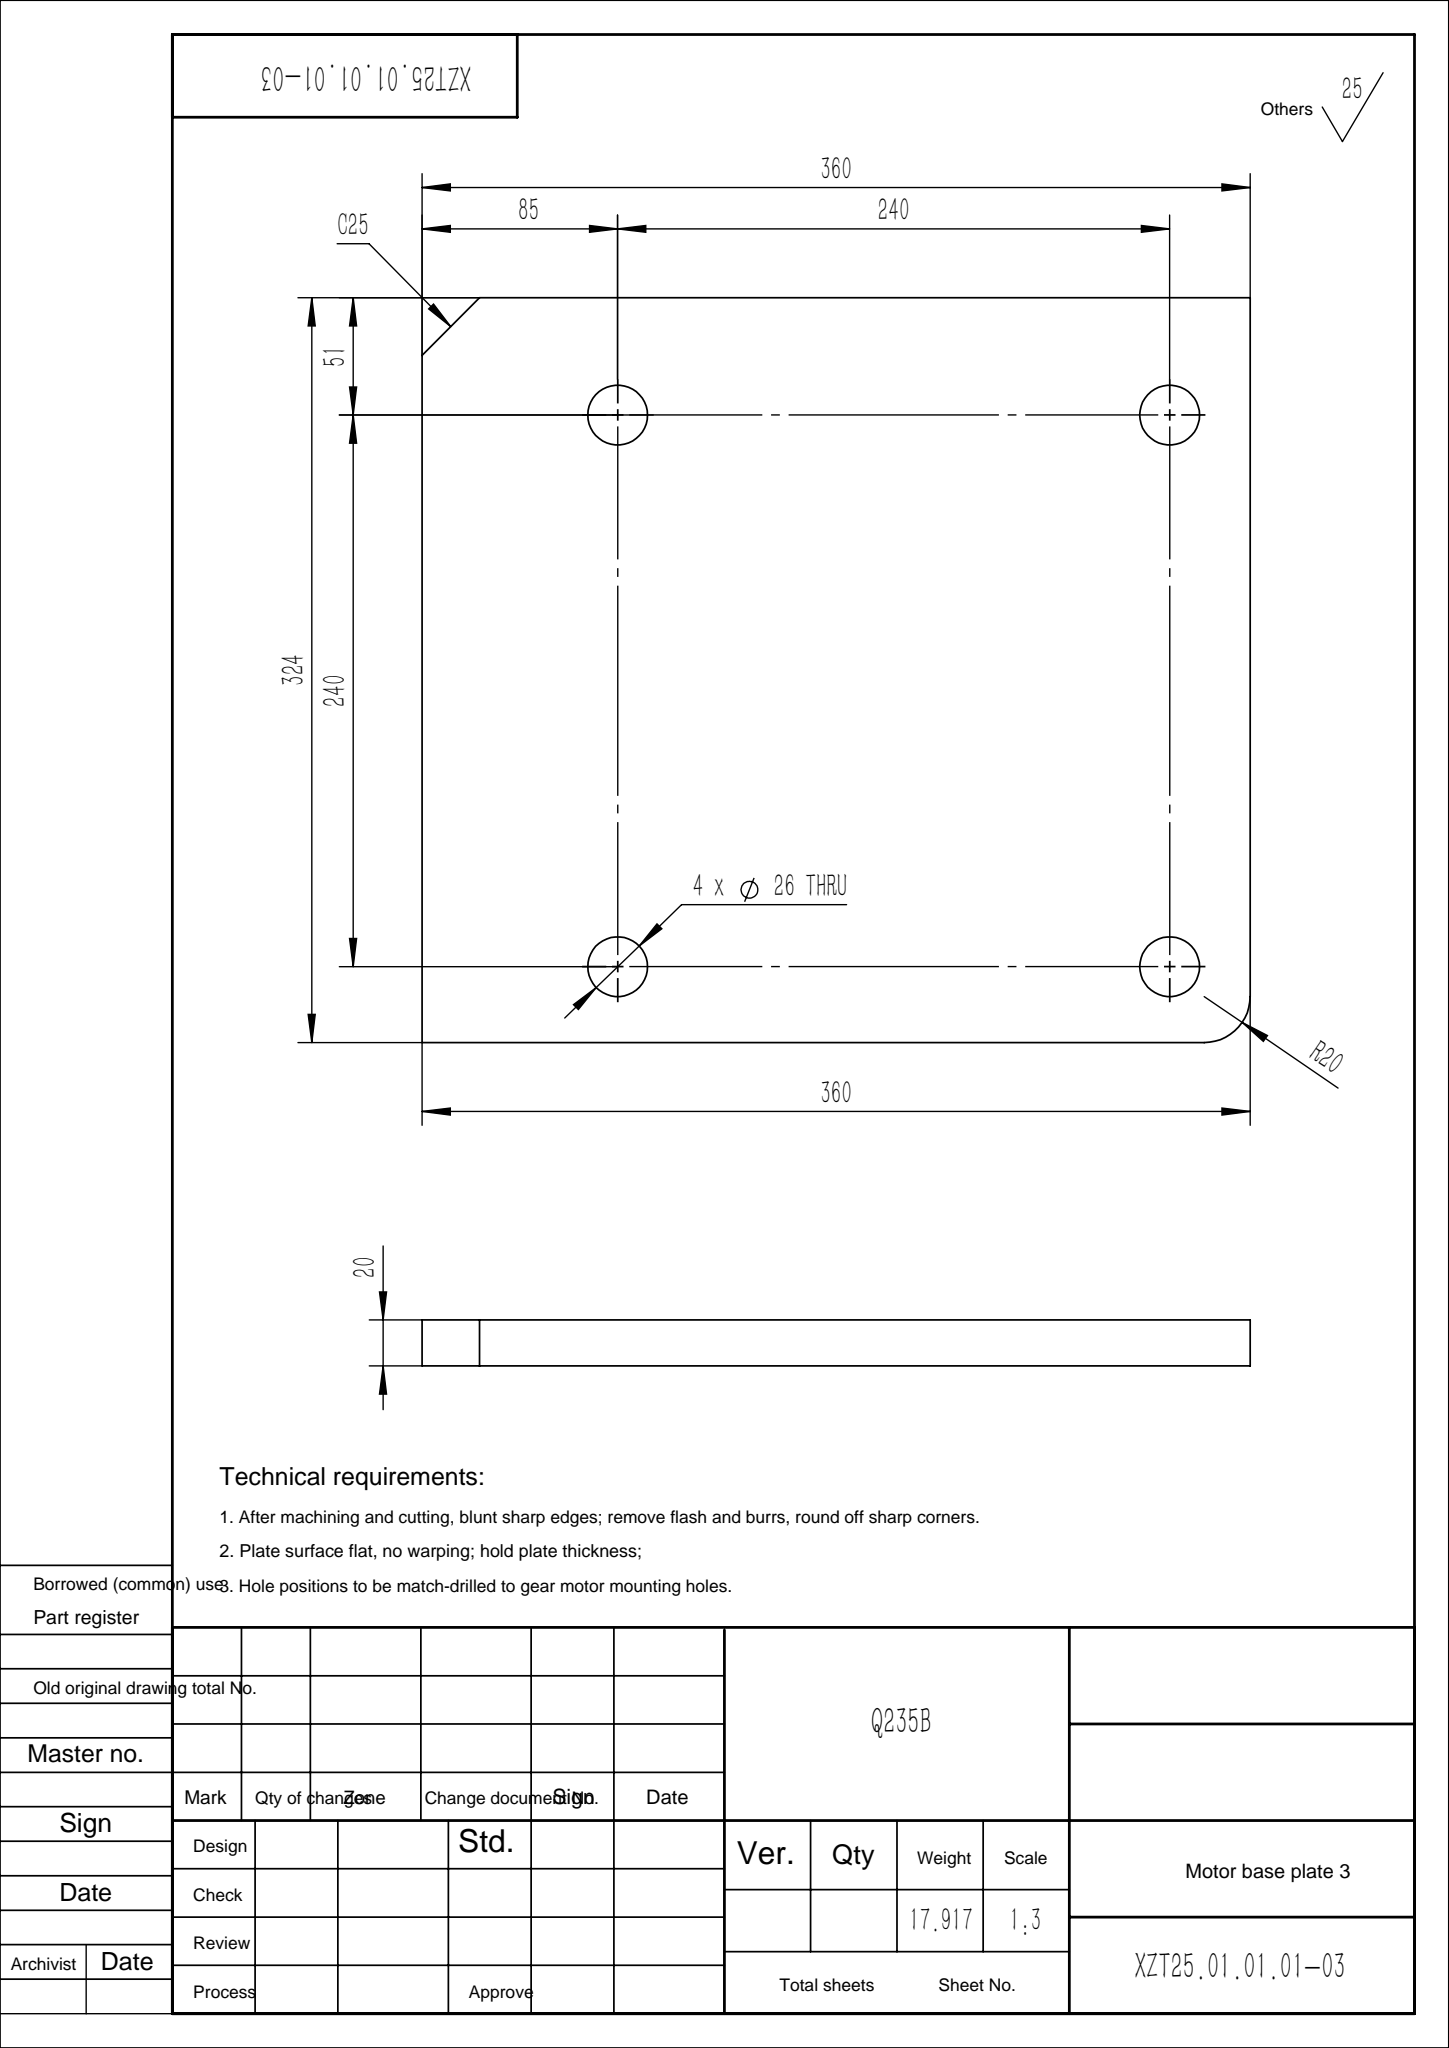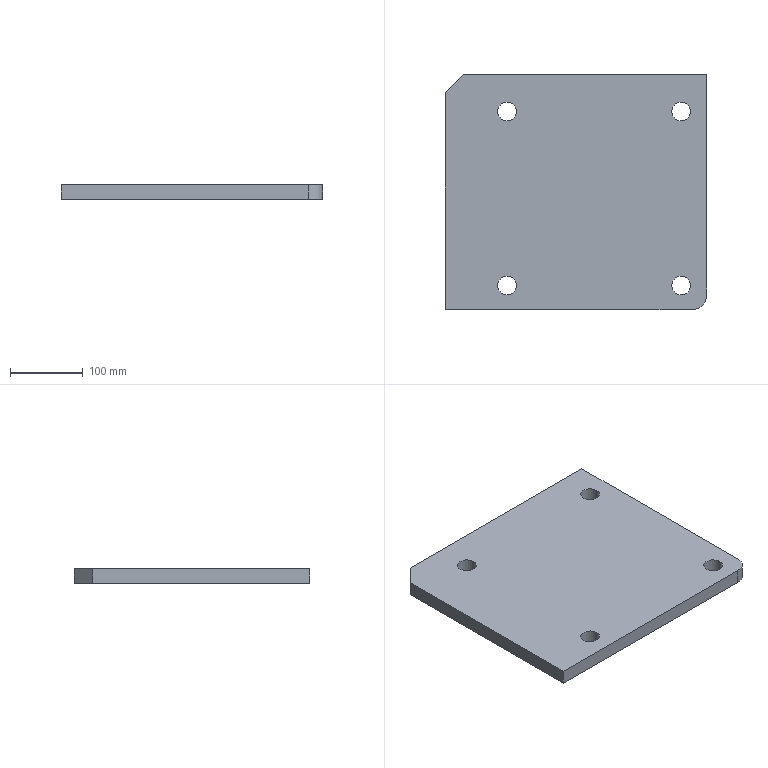Part | SolidWorks | features Chamfer 1, Extrusion 1, Fillet 1, HoleWzd 1 | 1 solid | 16 faces | box 360 x 324 x 20 mm | volume 2282359 mm3 | cylinder 9 | plane 7 | commonest cylinder face diameters 26 x8 40 x1
STEP:
#1=CARTESIAN_POINT('',(98.,33.,-10.));
#2=VERTEX_POINT('',#1);
#3=CARTESIAN_POINT('',(72.,33.,-10.));
#4=VERTEX_POINT('',#3);
#5=CARTESIAN_POINT('',(85.,33.,-10.));
#6=DIRECTION('',(0.,0.,-1.));
#7=DIRECTION('',(-1.,0.,0.));
#8=AXIS2_PLACEMENT_3D('',#5,#6,#7);
#9=CIRCLE('',#8,13.);
#10=EDGE_CURVE('',#2,#4,#9,.T.);
#11=ORIENTED_EDGE('',*,*,#10,.T.);
#12=CARTESIAN_POINT('',(72.,33.,10.));
#13=VERTEX_POINT('',#12);
#14=CARTESIAN_POINT('',(72.,33.,10.));
#15=DIRECTION('',(0.,0.,1.));
#16=VECTOR('',#15,1000.);
#17=LINE('',#14,#16);
#18=EDGE_CURVE('',#4,#13,#17,.T.);
#19=ORIENTED_EDGE('',*,*,#18,.T.);
#20=CARTESIAN_POINT('',(98.,33.,10.));
#21=VERTEX_POINT('',#20);
#22=CARTESIAN_POINT('',(85.,33.,10.));
#23=DIRECTION('',(0.,0.,1.));
#24=DIRECTION('',(1.,0.,0.));
#25=AXIS2_PLACEMENT_3D('',#22,#23,#24);
#26=CIRCLE('',#25,13.);
#27=EDGE_CURVE('',#13,#21,#26,.T.);
#28=ORIENTED_EDGE('',*,*,#27,.T.);
#29=CARTESIAN_POINT('',(98.,33.,10.));
#30=DIRECTION('',(0.,0.,1.));
#31=VECTOR('',#30,1000.);
#32=LINE('',#29,#31);
#33=EDGE_CURVE('',#2,#21,#32,.T.);
#34=ORIENTED_EDGE('',*,*,#33,.F.);
#35=EDGE_LOOP('',(#11,#19,#28,#34));
#36=FACE_OUTER_BOUND('',#35,.T.);
#37=CARTESIAN_POINT('',(85.,33.,10.));
#38=DIRECTION('',(0.,0.,1.));
#39=DIRECTION('',(1.,0.,0.));
#40=AXIS2_PLACEMENT_3D('',#37,#38,#39);
#41=CYLINDRICAL_SURFACE('',#40,13.);
#42=ADVANCED_FACE('',(#36),#41,.F.);
#43=CARTESIAN_POINT('',(338.,33.,-10.));
#44=VERTEX_POINT('',#43);
#45=CARTESIAN_POINT('',(312.,33.,-10.));
#46=VERTEX_POINT('',#45);
#47=CARTESIAN_POINT('',(325.,33.,-10.));
#48=DIRECTION('',(0.,0.,-1.));
#49=DIRECTION('',(-1.,0.,0.));
#50=AXIS2_PLACEMENT_3D('',#47,#48,#49);
#51=CIRCLE('',#50,13.);
#52=EDGE_CURVE('',#44,#46,#51,.T.);
#53=ORIENTED_EDGE('',*,*,#52,.T.);
#54=CARTESIAN_POINT('',(312.,33.,10.));
#55=VERTEX_POINT('',#54);
#56=CARTESIAN_POINT('',(312.,33.,10.));
#57=DIRECTION('',(0.,0.,1.));
#58=VECTOR('',#57,1000.);
#59=LINE('',#56,#58);
#60=EDGE_CURVE('',#46,#55,#59,.T.);
#61=ORIENTED_EDGE('',*,*,#60,.T.);
#62=CARTESIAN_POINT('',(338.,33.,10.));
#63=VERTEX_POINT('',#62);
#64=CARTESIAN_POINT('',(325.,33.,10.));
#65=DIRECTION('',(0.,0.,1.));
#66=DIRECTION('',(1.,0.,0.));
#67=AXIS2_PLACEMENT_3D('',#64,#65,#66);
#68=CIRCLE('',#67,13.);
#69=EDGE_CURVE('',#55,#63,#68,.T.);
#70=ORIENTED_EDGE('',*,*,#69,.T.);
#71=CARTESIAN_POINT('',(338.,33.,10.));
#72=DIRECTION('',(0.,0.,1.));
#73=VECTOR('',#72,1000.);
#74=LINE('',#71,#73);
#75=EDGE_CURVE('',#44,#63,#74,.T.);
#76=ORIENTED_EDGE('',*,*,#75,.F.);
#77=EDGE_LOOP('',(#53,#61,#70,#76));
#78=FACE_OUTER_BOUND('',#77,.T.);
#79=CARTESIAN_POINT('',(325.,33.,10.));
#80=DIRECTION('',(0.,0.,1.));
#81=DIRECTION('',(1.,0.,0.));
#82=AXIS2_PLACEMENT_3D('',#79,#80,#81);
#83=CYLINDRICAL_SURFACE('',#82,13.);
#84=ADVANCED_FACE('',(#78),#83,.F.);
#85=CARTESIAN_POINT('',(338.,273.,-10.));
#86=VERTEX_POINT('',#85);
#87=CARTESIAN_POINT('',(312.,273.,-10.));
#88=VERTEX_POINT('',#87);
#89=CARTESIAN_POINT('',(325.,273.,-10.));
#90=DIRECTION('',(0.,0.,-1.));
#91=DIRECTION('',(-1.,0.,0.));
#92=AXIS2_PLACEMENT_3D('',#89,#90,#91);
#93=CIRCLE('',#92,13.);
#94=EDGE_CURVE('',#86,#88,#93,.T.);
#95=ORIENTED_EDGE('',*,*,#94,.T.);
#96=CARTESIAN_POINT('',(312.,273.,10.));
#97=VERTEX_POINT('',#96);
#98=CARTESIAN_POINT('',(312.,273.,10.));
#99=DIRECTION('',(0.,0.,1.));
#100=VECTOR('',#99,1000.);
#101=LINE('',#98,#100);
#102=EDGE_CURVE('',#88,#97,#101,.T.);
#103=ORIENTED_EDGE('',*,*,#102,.T.);
#104=CARTESIAN_POINT('',(338.,273.,10.));
#105=VERTEX_POINT('',#104);
#106=CARTESIAN_POINT('',(325.,273.,10.));
#107=DIRECTION('',(0.,0.,1.));
#108=DIRECTION('',(1.,0.,0.));
#109=AXIS2_PLACEMENT_3D('',#106,#107,#108);
#110=CIRCLE('',#109,13.);
#111=EDGE_CURVE('',#97,#105,#110,.T.);
#112=ORIENTED_EDGE('',*,*,#111,.T.);
#113=CARTESIAN_POINT('',(338.,273.,10.));
#114=DIRECTION('',(0.,0.,1.));
#115=VECTOR('',#114,1000.);
#116=LINE('',#113,#115);
#117=EDGE_CURVE('',#86,#105,#116,.T.);
#118=ORIENTED_EDGE('',*,*,#117,.F.);
#119=EDGE_LOOP('',(#95,#103,#112,#118));
#120=FACE_OUTER_BOUND('',#119,.T.);
#121=CARTESIAN_POINT('',(325.,273.,10.));
#122=DIRECTION('',(0.,0.,1.));
#123=DIRECTION('',(1.,0.,0.));
#124=AXIS2_PLACEMENT_3D('',#121,#122,#123);
#125=CYLINDRICAL_SURFACE('',#124,13.);
#126=ADVANCED_FACE('',(#120),#125,.F.);
#127=CARTESIAN_POINT('',(98.,273.,-10.));
#128=VERTEX_POINT('',#127);
#129=CARTESIAN_POINT('',(72.,273.,-10.));
#130=VERTEX_POINT('',#129);
#131=CARTESIAN_POINT('',(85.,273.,-10.));
#132=DIRECTION('',(0.,0.,-1.));
#133=DIRECTION('',(-1.,0.,0.));
#134=AXIS2_PLACEMENT_3D('',#131,#132,#133);
#135=CIRCLE('',#134,13.);
#136=EDGE_CURVE('',#128,#130,#135,.T.);
#137=ORIENTED_EDGE('',*,*,#136,.T.);
#138=CARTESIAN_POINT('',(72.,273.,10.));
#139=VERTEX_POINT('',#138);
#140=CARTESIAN_POINT('',(72.,273.,10.));
#141=DIRECTION('',(0.,0.,1.));
#142=VECTOR('',#141,1000.);
#143=LINE('',#140,#142);
#144=EDGE_CURVE('',#130,#139,#143,.T.);
#145=ORIENTED_EDGE('',*,*,#144,.T.);
#146=CARTESIAN_POINT('',(98.,273.,10.));
#147=VERTEX_POINT('',#146);
#148=CARTESIAN_POINT('',(85.,273.,10.));
#149=DIRECTION('',(0.,0.,1.));
#150=DIRECTION('',(1.,0.,0.));
#151=AXIS2_PLACEMENT_3D('',#148,#149,#150);
#152=CIRCLE('',#151,13.);
#153=EDGE_CURVE('',#139,#147,#152,.T.);
#154=ORIENTED_EDGE('',*,*,#153,.T.);
#155=CARTESIAN_POINT('',(98.,273.,10.));
#156=DIRECTION('',(0.,0.,1.));
#157=VECTOR('',#156,1000.);
#158=LINE('',#155,#157);
#159=EDGE_CURVE('',#128,#147,#158,.T.);
#160=ORIENTED_EDGE('',*,*,#159,.F.);
#161=EDGE_LOOP('',(#137,#145,#154,#160));
#162=FACE_OUTER_BOUND('',#161,.T.);
#163=CARTESIAN_POINT('',(85.,273.,10.));
#164=DIRECTION('',(0.,0.,1.));
#165=DIRECTION('',(1.,0.,0.));
#166=AXIS2_PLACEMENT_3D('',#163,#164,#165);
#167=CYLINDRICAL_SURFACE('',#166,13.);
#168=ADVANCED_FACE('',(#162),#167,.F.);
#169=CARTESIAN_POINT('',(325.,273.,10.));
#170=DIRECTION('',(0.,0.,1.));
#171=DIRECTION('',(1.,0.,0.));
#172=AXIS2_PLACEMENT_3D('',#169,#170,#171);
#173=CIRCLE('',#172,13.);
#174=EDGE_CURVE('',#105,#97,#173,.T.);
#175=ORIENTED_EDGE('',*,*,#174,.F.);
#176=ORIENTED_EDGE('',*,*,#111,.F.);
#177=EDGE_LOOP('',(#175,#176));
#178=FACE_BOUND('',#177,.T.);
#179=CARTESIAN_POINT('',(85.,273.,10.));
#180=DIRECTION('',(0.,0.,1.));
#181=DIRECTION('',(1.,0.,0.));
#182=AXIS2_PLACEMENT_3D('',#179,#180,#181);
#183=CIRCLE('',#182,13.);
#184=EDGE_CURVE('',#147,#139,#183,.T.);
#185=ORIENTED_EDGE('',*,*,#184,.F.);
#186=ORIENTED_EDGE('',*,*,#153,.F.);
#187=EDGE_LOOP('',(#185,#186));
#188=FACE_BOUND('',#187,.T.);
#189=CARTESIAN_POINT('',(0.,0.,10.));
#190=VERTEX_POINT('',#189);
#191=CARTESIAN_POINT('',(340.,0.,10.));
#192=VERTEX_POINT('',#191);
#193=CARTESIAN_POINT('',(0.,0.,10.));
#194=DIRECTION('',(1.,0.,0.));
#195=VECTOR('',#194,1000.);
#196=LINE('',#193,#195);
#197=EDGE_CURVE('',#190,#192,#196,.T.);
#198=ORIENTED_EDGE('',*,*,#197,.T.);
#199=CARTESIAN_POINT('',(360.,20.,10.));
#200=VERTEX_POINT('',#199);
#201=CARTESIAN_POINT('',(340.,20.,10.));
#202=DIRECTION('',(0.,0.,1.));
#203=DIRECTION('',(-1.,0.,0.));
#204=AXIS2_PLACEMENT_3D('',#201,#202,#203);
#205=CIRCLE('',#204,20.);
#206=EDGE_CURVE('',#192,#200,#205,.T.);
#207=ORIENTED_EDGE('',*,*,#206,.T.);
#208=CARTESIAN_POINT('',(360.,324.,10.));
#209=VERTEX_POINT('',#208);
#210=CARTESIAN_POINT('',(360.,0.,10.));
#211=DIRECTION('',(0.,1.,0.));
#212=VECTOR('',#211,1000.);
#213=LINE('',#210,#212);
#214=EDGE_CURVE('',#200,#209,#213,.T.);
#215=ORIENTED_EDGE('',*,*,#214,.T.);
#216=CARTESIAN_POINT('',(25.,324.,10.));
#217=VERTEX_POINT('',#216);
#218=CARTESIAN_POINT('',(0.,324.,10.));
#219=DIRECTION('',(-1.,0.,0.));
#220=VECTOR('',#219,1000.);
#221=LINE('',#218,#220);
#222=EDGE_CURVE('',#209,#217,#221,.T.);
#223=ORIENTED_EDGE('',*,*,#222,.T.);
#224=CARTESIAN_POINT('',(0.,299.,10.));
#225=VERTEX_POINT('',#224);
#226=CARTESIAN_POINT('',(0.,299.,10.));
#227=DIRECTION('',(-0.7071,-0.7071,0.));
#228=VECTOR('',#227,1000.);
#229=LINE('',#226,#228);
#230=EDGE_CURVE('',#217,#225,#229,.T.);
#231=ORIENTED_EDGE('',*,*,#230,.T.);
#232=CARTESIAN_POINT('',(0.,0.,10.));
#233=DIRECTION('',(0.,-1.,0.));
#234=VECTOR('',#233,1000.);
#235=LINE('',#232,#234);
#236=EDGE_CURVE('',#225,#190,#235,.T.);
#237=ORIENTED_EDGE('',*,*,#236,.T.);
#238=EDGE_LOOP('',(#198,#207,#215,#223,#231,#237));
#239=FACE_OUTER_BOUND('',#238,.T.);
#240=CARTESIAN_POINT('',(325.,33.,10.));
#241=DIRECTION('',(0.,0.,1.));
#242=DIRECTION('',(1.,0.,0.));
#243=AXIS2_PLACEMENT_3D('',#240,#241,#242);
#244=CIRCLE('',#243,13.);
#245=EDGE_CURVE('',#63,#55,#244,.T.);
#246=ORIENTED_EDGE('',*,*,#245,.F.);
#247=ORIENTED_EDGE('',*,*,#69,.F.);
#248=EDGE_LOOP('',(#246,#247));
#249=FACE_BOUND('',#248,.T.);
#250=CARTESIAN_POINT('',(85.,33.,10.));
#251=DIRECTION('',(0.,0.,1.));
#252=DIRECTION('',(1.,0.,0.));
#253=AXIS2_PLACEMENT_3D('',#250,#251,#252);
#254=CIRCLE('',#253,13.);
#255=EDGE_CURVE('',#21,#13,#254,.T.);
#256=ORIENTED_EDGE('',*,*,#255,.F.);
#257=ORIENTED_EDGE('',*,*,#27,.F.);
#258=EDGE_LOOP('',(#256,#257));
#259=FACE_BOUND('',#258,.T.);
#260=CARTESIAN_POINT('',(0.,0.,10.));
#261=DIRECTION('',(0.,0.,-1.));
#262=DIRECTION('',(-1.,0.,0.));
#263=AXIS2_PLACEMENT_3D('',#260,#261,#262);
#264=PLANE('',#263);
#265=ADVANCED_FACE('',(#178,#188,#239,#249,#259),#264,.F.);
#266=ORIENTED_EDGE('',*,*,#236,.F.);
#267=CARTESIAN_POINT('',(0.,299.,-10.));
#268=VERTEX_POINT('',#267);
#269=CARTESIAN_POINT('',(0.,299.,10.));
#270=DIRECTION('',(0.,0.,-1.));
#271=VECTOR('',#270,1000.);
#272=LINE('',#269,#271);
#273=EDGE_CURVE('',#225,#268,#272,.T.);
#274=ORIENTED_EDGE('',*,*,#273,.T.);
#275=CARTESIAN_POINT('',(0.,0.,-10.));
#276=VERTEX_POINT('',#275);
#277=CARTESIAN_POINT('',(0.,0.,-10.));
#278=DIRECTION('',(0.,-1.,0.));
#279=VECTOR('',#278,1000.);
#280=LINE('',#277,#279);
#281=EDGE_CURVE('',#268,#276,#280,.T.);
#282=ORIENTED_EDGE('',*,*,#281,.T.);
#283=CARTESIAN_POINT('',(0.,0.,10.));
#284=DIRECTION('',(0.,0.,-1.));
#285=VECTOR('',#284,1000.);
#286=LINE('',#283,#285);
#287=EDGE_CURVE('',#190,#276,#286,.T.);
#288=ORIENTED_EDGE('',*,*,#287,.F.);
#289=EDGE_LOOP('',(#266,#274,#282,#288));
#290=FACE_OUTER_BOUND('',#289,.T.);
#291=CARTESIAN_POINT('',(0.,0.,10.));
#292=DIRECTION('',(1.,0.,0.));
#293=DIRECTION('',(0.,0.,-1.));
#294=AXIS2_PLACEMENT_3D('',#291,#292,#293);
#295=PLANE('',#294);
#296=ADVANCED_FACE('',(#290),#295,.F.);
#297=CARTESIAN_POINT('',(340.,0.,-10.));
#298=VERTEX_POINT('',#297);
#299=CARTESIAN_POINT('',(0.,0.,-10.));
#300=DIRECTION('',(1.,0.,0.));
#301=VECTOR('',#300,1000.);
#302=LINE('',#299,#301);
#303=EDGE_CURVE('',#276,#298,#302,.T.);
#304=ORIENTED_EDGE('',*,*,#303,.T.);
#305=CARTESIAN_POINT('',(340.,0.,10.));
#306=DIRECTION('',(0.,0.,1.));
#307=VECTOR('',#306,1000.);
#308=LINE('',#305,#307);
#309=EDGE_CURVE('',#298,#192,#308,.T.);
#310=ORIENTED_EDGE('',*,*,#309,.T.);
#311=ORIENTED_EDGE('',*,*,#197,.F.);
#312=ORIENTED_EDGE('',*,*,#287,.T.);
#313=EDGE_LOOP('',(#304,#310,#311,#312));
#314=FACE_OUTER_BOUND('',#313,.T.);
#315=CARTESIAN_POINT('',(0.,0.,10.));
#316=DIRECTION('',(0.,1.,0.));
#317=DIRECTION('',(0.,0.,1.));
#318=AXIS2_PLACEMENT_3D('',#315,#316,#317);
#319=PLANE('',#318);
#320=ADVANCED_FACE('',(#314),#319,.F.);
#321=ORIENTED_EDGE('',*,*,#214,.F.);
#322=CARTESIAN_POINT('',(360.,20.,-10.));
#323=VERTEX_POINT('',#322);
#324=CARTESIAN_POINT('',(360.,20.,10.));
#325=DIRECTION('',(0.,0.,-1.));
#326=VECTOR('',#325,1000.);
#327=LINE('',#324,#326);
#328=EDGE_CURVE('',#200,#323,#327,.T.);
#329=ORIENTED_EDGE('',*,*,#328,.T.);
#330=CARTESIAN_POINT('',(360.,324.,-10.));
#331=VERTEX_POINT('',#330);
#332=CARTESIAN_POINT('',(360.,0.,-10.));
#333=DIRECTION('',(0.,1.,0.));
#334=VECTOR('',#333,1000.);
#335=LINE('',#332,#334);
#336=EDGE_CURVE('',#323,#331,#335,.T.);
#337=ORIENTED_EDGE('',*,*,#336,.T.);
#338=CARTESIAN_POINT('',(360.,324.,10.));
#339=DIRECTION('',(0.,0.,-1.));
#340=VECTOR('',#339,1000.);
#341=LINE('',#338,#340);
#342=EDGE_CURVE('',#209,#331,#341,.T.);
#343=ORIENTED_EDGE('',*,*,#342,.F.);
#344=EDGE_LOOP('',(#321,#329,#337,#343));
#345=FACE_OUTER_BOUND('',#344,.T.);
#346=CARTESIAN_POINT('',(360.,0.,10.));
#347=DIRECTION('',(-1.,0.,0.));
#348=DIRECTION('',(0.,0.,1.));
#349=AXIS2_PLACEMENT_3D('',#346,#347,#348);
#350=PLANE('',#349);
#351=ADVANCED_FACE('',(#345),#350,.F.);
#352=CARTESIAN_POINT('',(25.,324.,-10.));
#353=VERTEX_POINT('',#352);
#354=CARTESIAN_POINT('',(0.,324.,-10.));
#355=DIRECTION('',(-1.,0.,0.));
#356=VECTOR('',#355,1000.);
#357=LINE('',#354,#356);
#358=EDGE_CURVE('',#331,#353,#357,.T.);
#359=ORIENTED_EDGE('',*,*,#358,.T.);
#360=CARTESIAN_POINT('',(25.,324.,10.));
#361=DIRECTION('',(0.,0.,1.));
#362=VECTOR('',#361,1000.);
#363=LINE('',#360,#362);
#364=EDGE_CURVE('',#353,#217,#363,.T.);
#365=ORIENTED_EDGE('',*,*,#364,.T.);
#366=ORIENTED_EDGE('',*,*,#222,.F.);
#367=ORIENTED_EDGE('',*,*,#342,.T.);
#368=EDGE_LOOP('',(#359,#365,#366,#367));
#369=FACE_OUTER_BOUND('',#368,.T.);
#370=CARTESIAN_POINT('',(0.,324.,10.));
#371=DIRECTION('',(0.,-1.,0.));
#372=DIRECTION('',(0.,0.,-1.));
#373=AXIS2_PLACEMENT_3D('',#370,#371,#372);
#374=PLANE('',#373);
#375=ADVANCED_FACE('',(#369),#374,.F.);
#376=ORIENTED_EDGE('',*,*,#10,.F.);
#377=CARTESIAN_POINT('',(85.,33.,-10.));
#378=DIRECTION('',(0.,0.,-1.));
#379=DIRECTION('',(-1.,0.,0.));
#380=AXIS2_PLACEMENT_3D('',#377,#378,#379);
#381=CIRCLE('',#380,13.);
#382=EDGE_CURVE('',#4,#2,#381,.T.);
#383=ORIENTED_EDGE('',*,*,#382,.F.);
#384=EDGE_LOOP('',(#376,#383));
#385=FACE_BOUND('',#384,.T.);
#386=ORIENTED_EDGE('',*,*,#52,.F.);
#387=CARTESIAN_POINT('',(325.,33.,-10.));
#388=DIRECTION('',(0.,0.,-1.));
#389=DIRECTION('',(-1.,0.,0.));
#390=AXIS2_PLACEMENT_3D('',#387,#388,#389);
#391=CIRCLE('',#390,13.);
#392=EDGE_CURVE('',#46,#44,#391,.T.);
#393=ORIENTED_EDGE('',*,*,#392,.F.);
#394=EDGE_LOOP('',(#386,#393));
#395=FACE_BOUND('',#394,.T.);
#396=ORIENTED_EDGE('',*,*,#94,.F.);
#397=CARTESIAN_POINT('',(325.,273.,-10.));
#398=DIRECTION('',(0.,0.,-1.));
#399=DIRECTION('',(-1.,0.,0.));
#400=AXIS2_PLACEMENT_3D('',#397,#398,#399);
#401=CIRCLE('',#400,13.);
#402=EDGE_CURVE('',#88,#86,#401,.T.);
#403=ORIENTED_EDGE('',*,*,#402,.F.);
#404=EDGE_LOOP('',(#396,#403));
#405=FACE_BOUND('',#404,.T.);
#406=ORIENTED_EDGE('',*,*,#136,.F.);
#407=CARTESIAN_POINT('',(85.,273.,-10.));
#408=DIRECTION('',(0.,0.,-1.));
#409=DIRECTION('',(-1.,0.,0.));
#410=AXIS2_PLACEMENT_3D('',#407,#408,#409);
#411=CIRCLE('',#410,13.);
#412=EDGE_CURVE('',#130,#128,#411,.T.);
#413=ORIENTED_EDGE('',*,*,#412,.F.);
#414=EDGE_LOOP('',(#406,#413));
#415=FACE_BOUND('',#414,.T.);
#416=ORIENTED_EDGE('',*,*,#336,.F.);
#417=CARTESIAN_POINT('',(340.,20.,-10.));
#418=DIRECTION('',(0.,0.,-1.));
#419=DIRECTION('',(-1.,0.,0.));
#420=AXIS2_PLACEMENT_3D('',#417,#418,#419);
#421=CIRCLE('',#420,20.);
#422=EDGE_CURVE('',#323,#298,#421,.T.);
#423=ORIENTED_EDGE('',*,*,#422,.T.);
#424=ORIENTED_EDGE('',*,*,#303,.F.);
#425=ORIENTED_EDGE('',*,*,#281,.F.);
#426=CARTESIAN_POINT('',(-149.5,149.5,-10.));
#427=DIRECTION('',(0.7071,0.7071,0.));
#428=VECTOR('',#427,1000.);
#429=LINE('',#426,#428);
#430=EDGE_CURVE('',#268,#353,#429,.T.);
#431=ORIENTED_EDGE('',*,*,#430,.T.);
#432=ORIENTED_EDGE('',*,*,#358,.F.);
#433=EDGE_LOOP('',(#416,#423,#424,#425,#431,#432));
#434=FACE_OUTER_BOUND('',#433,.T.);
#435=CARTESIAN_POINT('',(0.,0.,-10.));
#436=DIRECTION('',(0.,0.,-1.));
#437=DIRECTION('',(-1.,0.,0.));
#438=AXIS2_PLACEMENT_3D('',#435,#436,#437);
#439=PLANE('',#438);
#440=ADVANCED_FACE('',(#385,#395,#405,#415,#434),#439,.T.);
#441=ORIENTED_EDGE('',*,*,#230,.F.);
#442=ORIENTED_EDGE('',*,*,#364,.F.);
#443=ORIENTED_EDGE('',*,*,#430,.F.);
#444=ORIENTED_EDGE('',*,*,#273,.F.);
#445=EDGE_LOOP('',(#441,#442,#443,#444));
#446=FACE_OUTER_BOUND('',#445,.T.);
#447=CARTESIAN_POINT('',(0.,299.,10.));
#448=DIRECTION('',(0.7071,-0.7071,0.));
#449=DIRECTION('',(0.,0.,-1.));
#450=AXIS2_PLACEMENT_3D('',#447,#448,#449);
#451=PLANE('',#450);
#452=ADVANCED_FACE('',(#446),#451,.F.);
#453=ORIENTED_EDGE('',*,*,#206,.F.);
#454=ORIENTED_EDGE('',*,*,#309,.F.);
#455=ORIENTED_EDGE('',*,*,#422,.F.);
#456=ORIENTED_EDGE('',*,*,#328,.F.);
#457=EDGE_LOOP('',(#453,#454,#455,#456));
#458=FACE_OUTER_BOUND('',#457,.T.);
#459=CARTESIAN_POINT('',(340.,20.,10.));
#460=DIRECTION('',(0.,0.,-1.));
#461=DIRECTION('',(-1.,0.,0.));
#462=AXIS2_PLACEMENT_3D('',#459,#460,#461);
#463=CYLINDRICAL_SURFACE('',#462,20.);
#464=ADVANCED_FACE('',(#458),#463,.T.);
#465=ORIENTED_EDGE('',*,*,#144,.F.);
#466=ORIENTED_EDGE('',*,*,#412,.T.);
#467=ORIENTED_EDGE('',*,*,#159,.T.);
#468=ORIENTED_EDGE('',*,*,#184,.T.);
#469=EDGE_LOOP('',(#465,#466,#467,#468));
#470=FACE_OUTER_BOUND('',#469,.T.);
#471=CARTESIAN_POINT('',(85.,273.,10.));
#472=DIRECTION('',(0.,0.,1.));
#473=DIRECTION('',(1.,0.,0.));
#474=AXIS2_PLACEMENT_3D('',#471,#472,#473);
#475=CYLINDRICAL_SURFACE('',#474,13.);
#476=ADVANCED_FACE('',(#470),#475,.F.);
#477=ORIENTED_EDGE('',*,*,#102,.F.);
#478=ORIENTED_EDGE('',*,*,#402,.T.);
#479=ORIENTED_EDGE('',*,*,#117,.T.);
#480=ORIENTED_EDGE('',*,*,#174,.T.);
#481=EDGE_LOOP('',(#477,#478,#479,#480));
#482=FACE_OUTER_BOUND('',#481,.T.);
#483=CARTESIAN_POINT('',(325.,273.,10.));
#484=DIRECTION('',(0.,0.,1.));
#485=DIRECTION('',(1.,0.,0.));
#486=AXIS2_PLACEMENT_3D('',#483,#484,#485);
#487=CYLINDRICAL_SURFACE('',#486,13.);
#488=ADVANCED_FACE('',(#482),#487,.F.);
#489=ORIENTED_EDGE('',*,*,#60,.F.);
#490=ORIENTED_EDGE('',*,*,#392,.T.);
#491=ORIENTED_EDGE('',*,*,#75,.T.);
#492=ORIENTED_EDGE('',*,*,#245,.T.);
#493=EDGE_LOOP('',(#489,#490,#491,#492));
#494=FACE_OUTER_BOUND('',#493,.T.);
#495=CARTESIAN_POINT('',(325.,33.,10.));
#496=DIRECTION('',(0.,0.,1.));
#497=DIRECTION('',(1.,0.,0.));
#498=AXIS2_PLACEMENT_3D('',#495,#496,#497);
#499=CYLINDRICAL_SURFACE('',#498,13.);
#500=ADVANCED_FACE('',(#494),#499,.F.);
#501=ORIENTED_EDGE('',*,*,#18,.F.);
#502=ORIENTED_EDGE('',*,*,#382,.T.);
#503=ORIENTED_EDGE('',*,*,#33,.T.);
#504=ORIENTED_EDGE('',*,*,#255,.T.);
#505=EDGE_LOOP('',(#501,#502,#503,#504));
#506=FACE_OUTER_BOUND('',#505,.T.);
#507=CARTESIAN_POINT('',(85.,33.,10.));
#508=DIRECTION('',(0.,0.,1.));
#509=DIRECTION('',(1.,0.,0.));
#510=AXIS2_PLACEMENT_3D('',#507,#508,#509);
#511=CYLINDRICAL_SURFACE('',#510,13.);
#512=ADVANCED_FACE('',(#506),#511,.F.);
#513=CLOSED_SHELL('',(#42,#84,#126,#168,#265,#296,#320,#351,#375,#440,#452,#464,#476,#488,#500,#512));
#514=MANIFOLD_SOLID_BREP('',#513);
#515=CARTESIAN_POINT('',(0.,0.,0.));
#516=DIRECTION('',(0.,0.,1.));
#517=DIRECTION('',(1.,0.,0.));
#518=AXIS2_PLACEMENT_3D('',#515,#516,#517);
#519=(LENGTH_UNIT()NAMED_UNIT(*)SI_UNIT(.MILLI.,.METRE.));
#520=UNCERTAINTY_MEASURE_WITH_UNIT(LENGTH_MEASURE(0.00001),#519,'','');
#521=(NAMED_UNIT(*)PLANE_ANGLE_UNIT()SI_UNIT($,.RADIAN.));
#522=(NAMED_UNIT(*)SI_UNIT($,.STERADIAN.)SOLID_ANGLE_UNIT());
#523=(GEOMETRIC_REPRESENTATION_CONTEXT(3)GLOBAL_UNCERTAINTY_ASSIGNED_CONTEXT((#520))GLOBAL_UNIT_ASSIGNED_CONTEXT((#519,#521,#522))REPRESENTATION_CONTEXT('',''));
#524=ADVANCED_BREP_SHAPE_REPRESENTATION('',(#514,#518),#523);